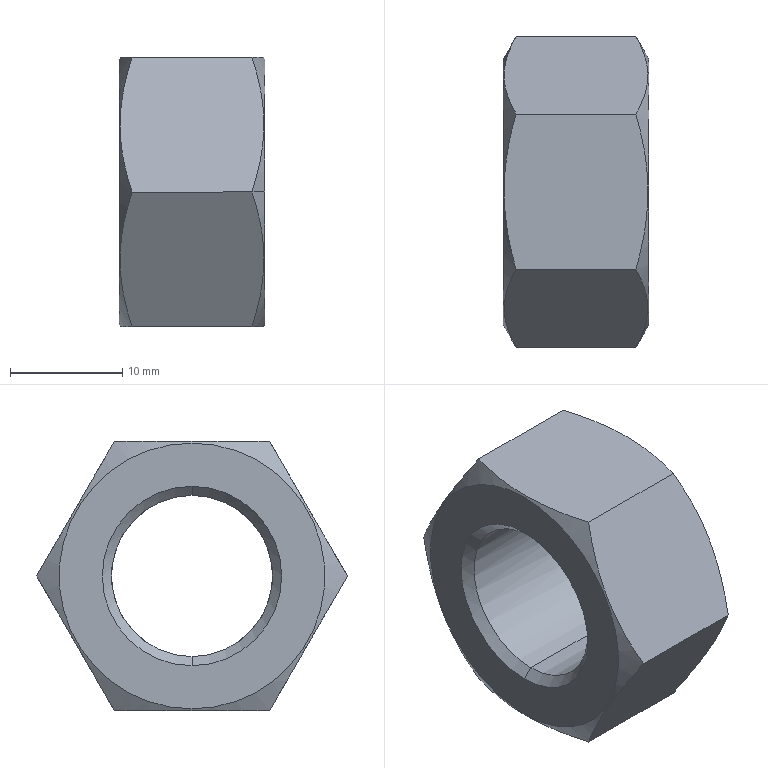Part | SolidWorks | features BaseBody 1 | 1 solid | 18 faces | box 13 x 27.713 x 24 mm | volume 4305 mm3 | cone 8 | plane 8 | cylinder 2 | commonest cylinder face diameters 14.376 x2
STEP:
#1=CARTESIAN_POINT('',(12.188,0.,-7.188));
#2=VERTEX_POINT('',#1);
#3=CARTESIAN_POINT('',(12.188,-7.188,0.));
#4=VERTEX_POINT('',#3);
#5=CARTESIAN_POINT('',(12.188,0.,0.));
#6=DIRECTION('',(-1.,0.,0.));
#7=DIRECTION('',(0.,0.,1.));
#8=AXIS2_PLACEMENT_3D('',#5,#6,#7);
#9=CIRCLE('',#8,7.188);
#10=EDGE_CURVE('',#2,#4,#9,.T.);
#11=ORIENTED_EDGE('',*,*,#10,.F.);
#12=CARTESIAN_POINT('',(0.812,0.,-7.188));
#13=VERTEX_POINT('',#12);
#14=CARTESIAN_POINT('',(13.,0.,-7.188));
#15=DIRECTION('',(-1.,0.,0.));
#16=VECTOR('',#15,1000.);
#17=LINE('',#14,#16);
#18=EDGE_CURVE('',#2,#13,#17,.T.);
#19=ORIENTED_EDGE('',*,*,#18,.T.);
#20=CARTESIAN_POINT('',(0.812,0.,7.188));
#21=VERTEX_POINT('',#20);
#22=CARTESIAN_POINT('',(0.812,0.,0.));
#23=DIRECTION('',(1.,0.,0.));
#24=DIRECTION('',(0.,0.,1.));
#25=AXIS2_PLACEMENT_3D('',#22,#23,#24);
#26=CIRCLE('',#25,7.188);
#27=EDGE_CURVE('',#21,#13,#26,.T.);
#28=ORIENTED_EDGE('',*,*,#27,.F.);
#29=CARTESIAN_POINT('',(12.188,0.,7.188));
#30=VERTEX_POINT('',#29);
#31=CARTESIAN_POINT('',(13.,0.,7.188));
#32=DIRECTION('',(-1.,0.,0.));
#33=VECTOR('',#32,1000.);
#34=LINE('',#31,#33);
#35=EDGE_CURVE('',#30,#21,#34,.T.);
#36=ORIENTED_EDGE('',*,*,#35,.F.);
#37=CARTESIAN_POINT('',(12.188,0.,0.));
#38=DIRECTION('',(-1.,0.,0.));
#39=DIRECTION('',(0.,0.,1.));
#40=AXIS2_PLACEMENT_3D('',#37,#38,#39);
#41=CIRCLE('',#40,7.188);
#42=EDGE_CURVE('',#4,#30,#41,.T.);
#43=ORIENTED_EDGE('',*,*,#42,.F.);
#44=EDGE_LOOP('',(#11,#19,#28,#36,#43));
#45=FACE_OUTER_BOUND('',#44,.T.);
#46=CARTESIAN_POINT('',(13.,0.,0.));
#47=DIRECTION('',(-1.,0.,0.));
#48=DIRECTION('',(0.,0.,1.));
#49=AXIS2_PLACEMENT_3D('',#46,#47,#48);
#50=CYLINDRICAL_SURFACE('',#49,7.188);
#51=ADVANCED_FACE('',(#45),#50,.F.);
#52=ORIENTED_EDGE('',*,*,#27,.T.);
#53=CARTESIAN_POINT('',(0.,0.,-8.));
#54=VERTEX_POINT('',#53);
#55=CARTESIAN_POINT('',(0.,0.,-8.));
#56=DIRECTION('',(-0.7071,0.,-0.7071));
#57=VECTOR('',#56,1000.);
#58=LINE('',#55,#57);
#59=EDGE_CURVE('',#13,#54,#58,.T.);
#60=ORIENTED_EDGE('',*,*,#59,.T.);
#61=CARTESIAN_POINT('',(0.,0.,8.));
#62=VERTEX_POINT('',#61);
#63=CARTESIAN_POINT('',(0.,0.,0.));
#64=DIRECTION('',(1.,0.,0.));
#65=DIRECTION('',(0.,0.,1.));
#66=AXIS2_PLACEMENT_3D('',#63,#64,#65);
#67=CIRCLE('',#66,8.);
#68=EDGE_CURVE('',#62,#54,#67,.T.);
#69=ORIENTED_EDGE('',*,*,#68,.F.);
#70=CARTESIAN_POINT('',(0.,0.,8.));
#71=DIRECTION('',(-0.7071,0.,0.7071));
#72=VECTOR('',#71,1000.);
#73=LINE('',#70,#72);
#74=EDGE_CURVE('',#21,#62,#73,.T.);
#75=ORIENTED_EDGE('',*,*,#74,.F.);
#76=EDGE_LOOP('',(#52,#60,#69,#75));
#77=FACE_OUTER_BOUND('',#76,.T.);
#78=CARTESIAN_POINT('',(0.,0.,0.));
#79=DIRECTION('',(-1.,0.,0.));
#80=DIRECTION('',(0.,0.,1.));
#81=AXIS2_PLACEMENT_3D('',#78,#79,#80);
#82=CONICAL_SURFACE('',#81,8.,0.7854);
#83=ADVANCED_FACE('',(#77),#82,.F.);
#84=CARTESIAN_POINT('',(12.188,7.188,0.));
#85=VERTEX_POINT('',#84);
#86=CARTESIAN_POINT('',(12.188,0.,0.));
#87=DIRECTION('',(-1.,0.,0.));
#88=DIRECTION('',(0.,0.,1.));
#89=AXIS2_PLACEMENT_3D('',#86,#87,#88);
#90=CIRCLE('',#89,7.188);
#91=EDGE_CURVE('',#85,#2,#90,.T.);
#92=ORIENTED_EDGE('',*,*,#91,.T.);
#93=ORIENTED_EDGE('',*,*,#10,.T.);
#94=CARTESIAN_POINT('',(13.,-8.,0.));
#95=VERTEX_POINT('',#94);
#96=CARTESIAN_POINT('',(13.,-8.,0.));
#97=DIRECTION('',(0.7071,-0.7071,0.));
#98=VECTOR('',#97,1000.);
#99=LINE('',#96,#98);
#100=EDGE_CURVE('',#4,#95,#99,.T.);
#101=ORIENTED_EDGE('',*,*,#100,.T.);
#102=CARTESIAN_POINT('',(13.,8.,0.));
#103=VERTEX_POINT('',#102);
#104=CARTESIAN_POINT('',(13.,0.,0.));
#105=DIRECTION('',(-1.,0.,0.));
#106=DIRECTION('',(0.,1.,0.));
#107=AXIS2_PLACEMENT_3D('',#104,#105,#106);
#108=CIRCLE('',#107,8.);
#109=EDGE_CURVE('',#103,#95,#108,.T.);
#110=ORIENTED_EDGE('',*,*,#109,.F.);
#111=CARTESIAN_POINT('',(13.,8.,0.));
#112=DIRECTION('',(0.7071,0.7071,0.));
#113=VECTOR('',#112,1000.);
#114=LINE('',#111,#113);
#115=EDGE_CURVE('',#85,#103,#114,.T.);
#116=ORIENTED_EDGE('',*,*,#115,.F.);
#117=EDGE_LOOP('',(#92,#93,#101,#110,#116));
#118=FACE_OUTER_BOUND('',#117,.T.);
#119=CARTESIAN_POINT('',(13.,0.,0.));
#120=DIRECTION('',(1.,0.,0.));
#121=DIRECTION('',(0.,1.,0.));
#122=AXIS2_PLACEMENT_3D('',#119,#120,#121);
#123=CONICAL_SURFACE('',#122,8.,0.7854);
#124=ADVANCED_FACE('',(#118),#123,.F.);
#125=CARTESIAN_POINT('',(0.,0.,-11.85));
#126=VERTEX_POINT('',#125);
#127=CARTESIAN_POINT('',(0.,0.,11.85));
#128=VERTEX_POINT('',#127);
#129=CARTESIAN_POINT('',(0.,0.,0.));
#130=DIRECTION('',(1.,0.,0.));
#131=DIRECTION('',(0.,0.,-1.));
#132=AXIS2_PLACEMENT_3D('',#129,#130,#131);
#133=CIRCLE('',#132,11.85);
#134=EDGE_CURVE('',#126,#128,#133,.T.);
#135=ORIENTED_EDGE('',*,*,#134,.T.);
#136=CARTESIAN_POINT('',(0.0866,0.,12.));
#137=VERTEX_POINT('',#136);
#138=CARTESIAN_POINT('',(1.165,0.,13.868));
#139=DIRECTION('',(0.5,0.,0.866));
#140=VECTOR('',#139,1000.);
#141=LINE('',#138,#140);
#142=EDGE_CURVE('',#128,#137,#141,.T.);
#143=ORIENTED_EDGE('',*,*,#142,.T.);
#144=CARTESIAN_POINT('',(1.158,6.928,12.));
#145=VERTEX_POINT('',#144);
#146=CARTESIAN_POINT('',(0.0866,0.,12.));
#147=CARTESIAN_POINT('',(0.0866,0.588,12.));
#148=CARTESIAN_POINT('',(0.1119,1.179,12.));
#149=CARTESIAN_POINT('',(0.21,2.347,12.));
#150=CARTESIAN_POINT('',(0.2826,2.927,12.));
#151=CARTESIAN_POINT('',(0.5626,4.658,12.));
#152=CARTESIAN_POINT('',(0.832,5.798,12.));
#153=CARTESIAN_POINT('',(1.158,6.928,12.));
#154=B_SPLINE_CURVE_WITH_KNOTS('',3,(#146,#147,#148,#149,#150,#151,#152,#153),.UNSPECIFIED.,.F.,.F.,(4,2,2,4),(0.00701,0.008756,0.0105,0.01399),.UNSPECIFIED.);
#155=EDGE_CURVE('',#137,#145,#154,.T.);
#156=ORIENTED_EDGE('',*,*,#155,.T.);
#157=CARTESIAN_POINT('',(1.158,13.856,0.000000037));
#158=VERTEX_POINT('',#157);
#159=CARTESIAN_POINT('',(1.158,6.928,12.));
#160=CARTESIAN_POINT('',(0.8318,7.494,11.02));
#161=CARTESIAN_POINT('',(0.5627,8.064,10.033));
#162=CARTESIAN_POINT('',(0.1898,9.215,8.039));
#163=CARTESIAN_POINT('',(0.08736,9.797,7.032));
#164=CARTESIAN_POINT('',(0.08623,10.68,5.501));
#165=CARTESIAN_POINT('',(0.1113,10.976,4.989));
#166=CARTESIAN_POINT('',(0.209,11.561,3.975));
#167=CARTESIAN_POINT('',(0.2815,11.852,3.472));
#168=CARTESIAN_POINT('',(0.5616,12.719,1.97));
#169=CARTESIAN_POINT('',(0.8314,13.29,0.9809));
#170=CARTESIAN_POINT('',(1.158,13.856,0.000000037));
#171=B_SPLINE_CURVE_WITH_KNOTS('',3,(#159,#160,#161,#162,#163,#164,#165,#166,#167,#168,#169,#170),.UNSPECIFIED.,.F.,.F.,(4,2,2,2,2,4),(0.,0.003499,0.006997,0.008746,0.0105,0.01399),.UNSPECIFIED.);
#172=EDGE_CURVE('',#145,#158,#171,.T.);
#173=ORIENTED_EDGE('',*,*,#172,.T.);
#174=CARTESIAN_POINT('',(1.158,6.928,-12.));
#175=VERTEX_POINT('',#174);
#176=CARTESIAN_POINT('',(1.158,13.856,0.000000037));
#177=CARTESIAN_POINT('',(0.8318,13.291,-0.9797));
#178=CARTESIAN_POINT('',(0.5627,12.721,-1.967));
#179=CARTESIAN_POINT('',(0.1898,11.57,-3.961));
#180=CARTESIAN_POINT('',(0.08736,10.988,-4.968));
#181=CARTESIAN_POINT('',(0.08623,10.104,-6.499));
#182=CARTESIAN_POINT('',(0.1113,9.809,-7.011));
#183=CARTESIAN_POINT('',(0.209,9.223,-8.025));
#184=CARTESIAN_POINT('',(0.2815,8.933,-8.528));
#185=CARTESIAN_POINT('',(0.5616,8.066,-10.03));
#186=CARTESIAN_POINT('',(0.8314,7.495,-11.019));
#187=CARTESIAN_POINT('',(1.158,6.928,-12.));
#188=B_SPLINE_CURVE_WITH_KNOTS('',3,(#176,#177,#178,#179,#180,#181,#182,#183,#184,#185,#186,#187),.UNSPECIFIED.,.F.,.F.,(4,2,2,2,2,4),(0.,0.003499,0.006997,0.008746,0.0105,0.01399),.UNSPECIFIED.);
#189=EDGE_CURVE('',#158,#175,#188,.T.);
#190=ORIENTED_EDGE('',*,*,#189,.T.);
#191=CARTESIAN_POINT('',(0.0866,0.,-12.));
#192=VERTEX_POINT('',#191);
#193=CARTESIAN_POINT('',(1.158,6.928,-12.));
#194=CARTESIAN_POINT('',(0.8312,5.795,-12.));
#195=CARTESIAN_POINT('',(0.5617,4.653,-12.));
#196=CARTESIAN_POINT('',(0.1888,2.346,-12.));
#197=CARTESIAN_POINT('',(0.0866,1.18,-12.));
#198=CARTESIAN_POINT('',(0.0866,0.,-12.));
#199=B_SPLINE_CURVE_WITH_KNOTS('',3,(#193,#194,#195,#196,#197,#198),.UNSPECIFIED.,.F.,.F.,(4,2,4),(0.,0.003505,0.00701),.UNSPECIFIED.);
#200=EDGE_CURVE('',#175,#192,#199,.T.);
#201=ORIENTED_EDGE('',*,*,#200,.T.);
#202=CARTESIAN_POINT('',(1.165,0.,-13.868));
#203=DIRECTION('',(0.5,0.,-0.866));
#204=VECTOR('',#203,1000.);
#205=LINE('',#202,#204);
#206=EDGE_CURVE('',#126,#192,#205,.T.);
#207=ORIENTED_EDGE('',*,*,#206,.F.);
#208=EDGE_LOOP('',(#135,#143,#156,#173,#190,#201,#207));
#209=FACE_OUTER_BOUND('',#208,.T.);
#210=CARTESIAN_POINT('',(1.165,0.,0.));
#211=DIRECTION('',(1.,0.,0.));
#212=DIRECTION('',(0.,0.,-1.));
#213=AXIS2_PLACEMENT_3D('',#210,#211,#212);
#214=CONICAL_SURFACE('',#213,13.868,1.047);
#215=ADVANCED_FACE('',(#209),#214,.T.);
#216=CARTESIAN_POINT('',(13.,-11.85,0.));
#217=VERTEX_POINT('',#216);
#218=CARTESIAN_POINT('',(13.,11.85,0.));
#219=VERTEX_POINT('',#218);
#220=CARTESIAN_POINT('',(13.,0.,0.));
#221=DIRECTION('',(-1.,0.,0.));
#222=DIRECTION('',(0.,-1.,0.));
#223=AXIS2_PLACEMENT_3D('',#220,#221,#222);
#224=CIRCLE('',#223,11.85);
#225=EDGE_CURVE('',#217,#219,#224,.T.);
#226=ORIENTED_EDGE('',*,*,#225,.T.);
#227=CARTESIAN_POINT('',(11.842,13.856,0.000000014));
#228=VERTEX_POINT('',#227);
#229=CARTESIAN_POINT('',(11.835,13.868,0.));
#230=DIRECTION('',(-0.5,0.866,0.));
#231=VECTOR('',#230,1000.);
#232=LINE('',#229,#231);
#233=EDGE_CURVE('',#219,#228,#232,.T.);
#234=ORIENTED_EDGE('',*,*,#233,.T.);
#235=CARTESIAN_POINT('',(11.842,6.928,12.));
#236=VERTEX_POINT('',#235);
#237=CARTESIAN_POINT('',(11.842,13.856,0.000000014));
#238=CARTESIAN_POINT('',(12.168,13.291,0.9797));
#239=CARTESIAN_POINT('',(12.437,12.721,1.967));
#240=CARTESIAN_POINT('',(12.81,11.57,3.961));
#241=CARTESIAN_POINT('',(12.913,10.988,4.968));
#242=CARTESIAN_POINT('',(12.914,10.104,6.499));
#243=CARTESIAN_POINT('',(12.889,9.809,7.011));
#244=CARTESIAN_POINT('',(12.791,9.223,8.025));
#245=CARTESIAN_POINT('',(12.718,8.933,8.528));
#246=CARTESIAN_POINT('',(12.438,8.066,10.03));
#247=CARTESIAN_POINT('',(12.169,7.495,11.019));
#248=CARTESIAN_POINT('',(11.842,6.928,12.));
#249=B_SPLINE_CURVE_WITH_KNOTS('',3,(#237,#238,#239,#240,#241,#242,#243,#244,#245,#246,#247,#248),.UNSPECIFIED.,.F.,.F.,(4,2,2,2,2,4),(0.,0.003499,0.006997,0.008746,0.0105,0.01399),.UNSPECIFIED.);
#250=EDGE_CURVE('',#228,#236,#249,.T.);
#251=ORIENTED_EDGE('',*,*,#250,.T.);
#252=CARTESIAN_POINT('',(11.842,-6.928,12.));
#253=VERTEX_POINT('',#252);
#254=CARTESIAN_POINT('',(11.842,6.928,12.));
#255=CARTESIAN_POINT('',(12.168,5.797,12.));
#256=CARTESIAN_POINT('',(12.437,4.657,12.));
#257=CARTESIAN_POINT('',(12.81,2.355,12.));
#258=CARTESIAN_POINT('',(12.913,1.191,12.));
#259=CARTESIAN_POINT('',(12.914,-0.5758,12.));
#260=CARTESIAN_POINT('',(12.889,-1.168,12.));
#261=CARTESIAN_POINT('',(12.791,-2.338,12.));
#262=CARTESIAN_POINT('',(12.718,-2.92,12.));
#263=CARTESIAN_POINT('',(12.438,-4.653,12.));
#264=CARTESIAN_POINT('',(12.169,-5.796,12.));
#265=CARTESIAN_POINT('',(11.842,-6.928,12.));
#266=B_SPLINE_CURVE_WITH_KNOTS('',3,(#254,#255,#256,#257,#258,#259,#260,#261,#262,#263,#264,#265),.UNSPECIFIED.,.F.,.F.,(4,2,2,2,2,4),(0.,0.003499,0.006997,0.008746,0.0105,0.01399),.UNSPECIFIED.);
#267=EDGE_CURVE('',#236,#253,#266,.T.);
#268=ORIENTED_EDGE('',*,*,#267,.T.);
#269=CARTESIAN_POINT('',(11.842,-13.856,0.000000012));
#270=VERTEX_POINT('',#269);
#271=CARTESIAN_POINT('',(11.842,-6.928,12.));
#272=CARTESIAN_POINT('',(12.168,-7.494,11.02));
#273=CARTESIAN_POINT('',(12.437,-8.064,10.033));
#274=CARTESIAN_POINT('',(12.81,-9.215,8.039));
#275=CARTESIAN_POINT('',(12.913,-9.797,7.032));
#276=CARTESIAN_POINT('',(12.914,-10.68,5.501));
#277=CARTESIAN_POINT('',(12.889,-10.976,4.989));
#278=CARTESIAN_POINT('',(12.791,-11.561,3.975));
#279=CARTESIAN_POINT('',(12.718,-11.852,3.472));
#280=CARTESIAN_POINT('',(12.438,-12.719,1.97));
#281=CARTESIAN_POINT('',(12.169,-13.29,0.9809));
#282=CARTESIAN_POINT('',(11.842,-13.856,0.000000012));
#283=B_SPLINE_CURVE_WITH_KNOTS('',3,(#271,#272,#273,#274,#275,#276,#277,#278,#279,#280,#281,#282),.UNSPECIFIED.,.F.,.F.,(4,2,2,2,2,4),(0.,0.003499,0.006997,0.008746,0.0105,0.01399),.UNSPECIFIED.);
#284=EDGE_CURVE('',#253,#270,#283,.T.);
#285=ORIENTED_EDGE('',*,*,#284,.T.);
#286=CARTESIAN_POINT('',(11.835,-13.868,0.));
#287=DIRECTION('',(-0.5,-0.866,0.));
#288=VECTOR('',#287,1000.);
#289=LINE('',#286,#288);
#290=EDGE_CURVE('',#217,#270,#289,.T.);
#291=ORIENTED_EDGE('',*,*,#290,.F.);
#292=EDGE_LOOP('',(#226,#234,#251,#268,#285,#291));
#293=FACE_OUTER_BOUND('',#292,.T.);
#294=CARTESIAN_POINT('',(11.835,0.,0.));
#295=DIRECTION('',(-1.,0.,0.));
#296=DIRECTION('',(0.,-1.,0.));
#297=AXIS2_PLACEMENT_3D('',#294,#295,#296);
#298=CONICAL_SURFACE('',#297,13.868,1.047);
#299=ADVANCED_FACE('',(#293),#298,.T.);
#300=ORIENTED_EDGE('',*,*,#18,.F.);
#301=ORIENTED_EDGE('',*,*,#91,.F.);
#302=CARTESIAN_POINT('',(12.188,0.,0.));
#303=DIRECTION('',(-1.,0.,0.));
#304=DIRECTION('',(0.,0.,1.));
#305=AXIS2_PLACEMENT_3D('',#302,#303,#304);
#306=CIRCLE('',#305,7.188);
#307=EDGE_CURVE('',#30,#85,#306,.T.);
#308=ORIENTED_EDGE('',*,*,#307,.F.);
#309=ORIENTED_EDGE('',*,*,#35,.T.);
#310=CARTESIAN_POINT('',(0.812,0.,0.));
#311=DIRECTION('',(1.,0.,0.));
#312=DIRECTION('',(0.,0.,1.));
#313=AXIS2_PLACEMENT_3D('',#310,#311,#312);
#314=CIRCLE('',#313,7.188);
#315=EDGE_CURVE('',#13,#21,#314,.T.);
#316=ORIENTED_EDGE('',*,*,#315,.F.);
#317=EDGE_LOOP('',(#300,#301,#308,#309,#316));
#318=FACE_OUTER_BOUND('',#317,.T.);
#319=CARTESIAN_POINT('',(13.,0.,0.));
#320=DIRECTION('',(-1.,0.,0.));
#321=DIRECTION('',(0.,0.,1.));
#322=AXIS2_PLACEMENT_3D('',#319,#320,#321);
#323=CYLINDRICAL_SURFACE('',#322,7.188);
#324=ADVANCED_FACE('',(#318),#323,.F.);
#325=ORIENTED_EDGE('',*,*,#59,.F.);
#326=ORIENTED_EDGE('',*,*,#315,.T.);
#327=ORIENTED_EDGE('',*,*,#74,.T.);
#328=CARTESIAN_POINT('',(0.,0.,0.));
#329=DIRECTION('',(1.,0.,0.));
#330=DIRECTION('',(0.,0.,1.));
#331=AXIS2_PLACEMENT_3D('',#328,#329,#330);
#332=CIRCLE('',#331,8.);
#333=EDGE_CURVE('',#54,#62,#332,.T.);
#334=ORIENTED_EDGE('',*,*,#333,.F.);
#335=EDGE_LOOP('',(#325,#326,#327,#334));
#336=FACE_OUTER_BOUND('',#335,.T.);
#337=CARTESIAN_POINT('',(0.,0.,0.));
#338=DIRECTION('',(-1.,0.,0.));
#339=DIRECTION('',(0.,0.,1.));
#340=AXIS2_PLACEMENT_3D('',#337,#338,#339);
#341=CONICAL_SURFACE('',#340,8.,0.7854);
#342=ADVANCED_FACE('',(#336),#341,.F.);
#343=ORIENTED_EDGE('',*,*,#100,.F.);
#344=ORIENTED_EDGE('',*,*,#42,.T.);
#345=ORIENTED_EDGE('',*,*,#307,.T.);
#346=ORIENTED_EDGE('',*,*,#115,.T.);
#347=CARTESIAN_POINT('',(13.,0.,0.));
#348=DIRECTION('',(-1.,0.,0.));
#349=DIRECTION('',(0.,1.,0.));
#350=AXIS2_PLACEMENT_3D('',#347,#348,#349);
#351=CIRCLE('',#350,8.);
#352=EDGE_CURVE('',#95,#103,#351,.T.);
#353=ORIENTED_EDGE('',*,*,#352,.F.);
#354=EDGE_LOOP('',(#343,#344,#345,#346,#353));
#355=FACE_OUTER_BOUND('',#354,.T.);
#356=CARTESIAN_POINT('',(13.,0.,0.));
#357=DIRECTION('',(1.,0.,0.));
#358=DIRECTION('',(0.,1.,0.));
#359=AXIS2_PLACEMENT_3D('',#356,#357,#358);
#360=CONICAL_SURFACE('',#359,8.,0.7854);
#361=ADVANCED_FACE('',(#355),#360,.F.);
#362=ORIENTED_EDGE('',*,*,#68,.T.);
#363=ORIENTED_EDGE('',*,*,#333,.T.);
#364=EDGE_LOOP('',(#362,#363));
#365=FACE_BOUND('',#364,.T.);
#366=ORIENTED_EDGE('',*,*,#134,.F.);
#367=CARTESIAN_POINT('',(0.,0.,0.));
#368=DIRECTION('',(1.,0.,0.));
#369=DIRECTION('',(0.,0.,-1.));
#370=AXIS2_PLACEMENT_3D('',#367,#368,#369);
#371=CIRCLE('',#370,11.85);
#372=EDGE_CURVE('',#128,#126,#371,.T.);
#373=ORIENTED_EDGE('',*,*,#372,.F.);
#374=EDGE_LOOP('',(#366,#373));
#375=FACE_OUTER_BOUND('',#374,.T.);
#376=CARTESIAN_POINT('',(0.,0.,0.));
#377=DIRECTION('',(1.,0.,0.));
#378=DIRECTION('',(0.,0.,-1.));
#379=AXIS2_PLACEMENT_3D('',#376,#377,#378);
#380=PLANE('',#379);
#381=ADVANCED_FACE('',(#365,#375),#380,.F.);
#382=ORIENTED_EDGE('',*,*,#225,.F.);
#383=CARTESIAN_POINT('',(13.,0.,0.));
#384=DIRECTION('',(-1.,0.,0.));
#385=DIRECTION('',(0.,-1.,0.));
#386=AXIS2_PLACEMENT_3D('',#383,#384,#385);
#387=CIRCLE('',#386,11.85);
#388=EDGE_CURVE('',#219,#217,#387,.T.);
#389=ORIENTED_EDGE('',*,*,#388,.F.);
#390=EDGE_LOOP('',(#382,#389));
#391=FACE_OUTER_BOUND('',#390,.T.);
#392=ORIENTED_EDGE('',*,*,#109,.T.);
#393=ORIENTED_EDGE('',*,*,#352,.T.);
#394=EDGE_LOOP('',(#392,#393));
#395=FACE_BOUND('',#394,.T.);
#396=CARTESIAN_POINT('',(13.,11.85,0.));
#397=DIRECTION('',(-1.,0.,0.));
#398=DIRECTION('',(0.,0.,1.));
#399=AXIS2_PLACEMENT_3D('',#396,#397,#398);
#400=PLANE('',#399);
#401=ADVANCED_FACE('',(#391,#395),#400,.F.);
#402=ORIENTED_EDGE('',*,*,#142,.F.);
#403=ORIENTED_EDGE('',*,*,#372,.T.);
#404=ORIENTED_EDGE('',*,*,#206,.T.);
#405=CARTESIAN_POINT('',(1.158,-6.928,-12.));
#406=VERTEX_POINT('',#405);
#407=CARTESIAN_POINT('',(0.0866,0.,-12.));
#408=CARTESIAN_POINT('',(0.0866,-0.588,-12.));
#409=CARTESIAN_POINT('',(0.1119,-1.179,-12.));
#410=CARTESIAN_POINT('',(0.21,-2.347,-12.));
#411=CARTESIAN_POINT('',(0.2826,-2.927,-12.));
#412=CARTESIAN_POINT('',(0.5626,-4.658,-12.));
#413=CARTESIAN_POINT('',(0.832,-5.798,-12.));
#414=CARTESIAN_POINT('',(1.158,-6.928,-12.));
#415=B_SPLINE_CURVE_WITH_KNOTS('',3,(#407,#408,#409,#410,#411,#412,#413,#414),.UNSPECIFIED.,.F.,.F.,(4,2,2,4),(0.00701,0.008756,0.0105,0.01399),.UNSPECIFIED.);
#416=EDGE_CURVE('',#192,#406,#415,.T.);
#417=ORIENTED_EDGE('',*,*,#416,.T.);
#418=CARTESIAN_POINT('',(1.158,-13.856,-0.000000037));
#419=VERTEX_POINT('',#418);
#420=CARTESIAN_POINT('',(1.158,-6.928,-12.));
#421=CARTESIAN_POINT('',(0.8318,-7.494,-11.02));
#422=CARTESIAN_POINT('',(0.5627,-8.064,-10.033));
#423=CARTESIAN_POINT('',(0.1898,-9.215,-8.039));
#424=CARTESIAN_POINT('',(0.08736,-9.797,-7.032));
#425=CARTESIAN_POINT('',(0.08623,-10.68,-5.501));
#426=CARTESIAN_POINT('',(0.1113,-10.976,-4.989));
#427=CARTESIAN_POINT('',(0.209,-11.561,-3.975));
#428=CARTESIAN_POINT('',(0.2815,-11.852,-3.472));
#429=CARTESIAN_POINT('',(0.5616,-12.719,-1.97));
#430=CARTESIAN_POINT('',(0.8314,-13.29,-0.9809));
#431=CARTESIAN_POINT('',(1.158,-13.856,-0.000000037));
#432=B_SPLINE_CURVE_WITH_KNOTS('',3,(#420,#421,#422,#423,#424,#425,#426,#427,#428,#429,#430,#431),.UNSPECIFIED.,.F.,.F.,(4,2,2,2,2,4),(0.,0.003499,0.006997,0.008746,0.0105,0.01399),.UNSPECIFIED.);
#433=EDGE_CURVE('',#406,#419,#432,.T.);
#434=ORIENTED_EDGE('',*,*,#433,.T.);
#435=CARTESIAN_POINT('',(1.158,-6.928,12.));
#436=VERTEX_POINT('',#435);
#437=CARTESIAN_POINT('',(1.158,-13.856,-0.000000037));
#438=CARTESIAN_POINT('',(0.8318,-13.291,0.9797));
#439=CARTESIAN_POINT('',(0.5627,-12.721,1.967));
#440=CARTESIAN_POINT('',(0.1898,-11.57,3.961));
#441=CARTESIAN_POINT('',(0.08736,-10.988,4.968));
#442=CARTESIAN_POINT('',(0.08623,-10.104,6.499));
#443=CARTESIAN_POINT('',(0.1113,-9.809,7.011));
#444=CARTESIAN_POINT('',(0.209,-9.223,8.025));
#445=CARTESIAN_POINT('',(0.2815,-8.933,8.528));
#446=CARTESIAN_POINT('',(0.5616,-8.066,10.03));
#447=CARTESIAN_POINT('',(0.8314,-7.495,11.019));
#448=CARTESIAN_POINT('',(1.158,-6.928,12.));
#449=B_SPLINE_CURVE_WITH_KNOTS('',3,(#437,#438,#439,#440,#441,#442,#443,#444,#445,#446,#447,#448),.UNSPECIFIED.,.F.,.F.,(4,2,2,2,2,4),(0.,0.003499,0.006997,0.008746,0.0105,0.01399),.UNSPECIFIED.);
#450=EDGE_CURVE('',#419,#436,#449,.T.);
#451=ORIENTED_EDGE('',*,*,#450,.T.);
#452=CARTESIAN_POINT('',(1.158,-6.928,12.));
#453=CARTESIAN_POINT('',(0.8312,-5.795,12.));
#454=CARTESIAN_POINT('',(0.5617,-4.653,12.));
#455=CARTESIAN_POINT('',(0.1888,-2.346,12.));
#456=CARTESIAN_POINT('',(0.0866,-1.18,12.));
#457=CARTESIAN_POINT('',(0.0866,0.,12.));
#458=B_SPLINE_CURVE_WITH_KNOTS('',3,(#452,#453,#454,#455,#456,#457),.UNSPECIFIED.,.F.,.F.,(4,2,4),(0.,0.003505,0.00701),.UNSPECIFIED.);
#459=EDGE_CURVE('',#436,#137,#458,.T.);
#460=ORIENTED_EDGE('',*,*,#459,.T.);
#461=EDGE_LOOP('',(#402,#403,#404,#417,#434,#451,#460));
#462=FACE_OUTER_BOUND('',#461,.T.);
#463=CARTESIAN_POINT('',(1.165,0.,0.));
#464=DIRECTION('',(1.,0.,0.));
#465=DIRECTION('',(0.,0.,-1.));
#466=AXIS2_PLACEMENT_3D('',#463,#464,#465);
#467=CONICAL_SURFACE('',#466,13.868,1.047);
#468=ADVANCED_FACE('',(#462),#467,.T.);
#469=ORIENTED_EDGE('',*,*,#233,.F.);
#470=ORIENTED_EDGE('',*,*,#388,.T.);
#471=ORIENTED_EDGE('',*,*,#290,.T.);
#472=CARTESIAN_POINT('',(11.842,-6.928,-12.));
#473=VERTEX_POINT('',#472);
#474=CARTESIAN_POINT('',(11.842,-13.856,0.000000012));
#475=CARTESIAN_POINT('',(12.168,-13.291,-0.9797));
#476=CARTESIAN_POINT('',(12.437,-12.721,-1.967));
#477=CARTESIAN_POINT('',(12.81,-11.57,-3.961));
#478=CARTESIAN_POINT('',(12.913,-10.988,-4.968));
#479=CARTESIAN_POINT('',(12.914,-10.104,-6.499));
#480=CARTESIAN_POINT('',(12.889,-9.809,-7.011));
#481=CARTESIAN_POINT('',(12.791,-9.223,-8.025));
#482=CARTESIAN_POINT('',(12.718,-8.933,-8.528));
#483=CARTESIAN_POINT('',(12.438,-8.066,-10.03));
#484=CARTESIAN_POINT('',(12.169,-7.495,-11.019));
#485=CARTESIAN_POINT('',(11.842,-6.928,-12.));
#486=B_SPLINE_CURVE_WITH_KNOTS('',3,(#474,#475,#476,#477,#478,#479,#480,#481,#482,#483,#484,#485),.UNSPECIFIED.,.F.,.F.,(4,2,2,2,2,4),(0.,0.003499,0.006997,0.008746,0.0105,0.01399),.UNSPECIFIED.);
#487=EDGE_CURVE('',#270,#473,#486,.T.);
#488=ORIENTED_EDGE('',*,*,#487,.T.);
#489=CARTESIAN_POINT('',(11.842,6.928,-12.));
#490=VERTEX_POINT('',#489);
#491=CARTESIAN_POINT('',(11.842,-6.928,-12.));
#492=CARTESIAN_POINT('',(12.168,-5.797,-12.));
#493=CARTESIAN_POINT('',(12.437,-4.657,-12.));
#494=CARTESIAN_POINT('',(12.81,-2.355,-12.));
#495=CARTESIAN_POINT('',(12.913,-1.191,-12.));
#496=CARTESIAN_POINT('',(12.914,0.5758,-12.));
#497=CARTESIAN_POINT('',(12.889,1.168,-12.));
#498=CARTESIAN_POINT('',(12.791,2.338,-12.));
#499=CARTESIAN_POINT('',(12.718,2.92,-12.));
#500=CARTESIAN_POINT('',(12.438,4.653,-12.));
#501=CARTESIAN_POINT('',(12.169,5.796,-12.));
#502=CARTESIAN_POINT('',(11.842,6.928,-12.));
#503=B_SPLINE_CURVE_WITH_KNOTS('',3,(#491,#492,#493,#494,#495,#496,#497,#498,#499,#500,#501,#502),.UNSPECIFIED.,.F.,.F.,(4,2,2,2,2,4),(0.,0.003499,0.006997,0.008746,0.0105,0.01399),.UNSPECIFIED.);
#504=EDGE_CURVE('',#473,#490,#503,.T.);
#505=ORIENTED_EDGE('',*,*,#504,.T.);
#506=CARTESIAN_POINT('',(11.842,6.928,-12.));
#507=CARTESIAN_POINT('',(12.168,7.494,-11.02));
#508=CARTESIAN_POINT('',(12.437,8.064,-10.033));
#509=CARTESIAN_POINT('',(12.81,9.215,-8.039));
#510=CARTESIAN_POINT('',(12.913,9.797,-7.032));
#511=CARTESIAN_POINT('',(12.914,10.68,-5.501));
#512=CARTESIAN_POINT('',(12.889,10.976,-4.989));
#513=CARTESIAN_POINT('',(12.791,11.561,-3.975));
#514=CARTESIAN_POINT('',(12.718,11.852,-3.472));
#515=CARTESIAN_POINT('',(12.438,12.719,-1.97));
#516=CARTESIAN_POINT('',(12.169,13.29,-0.9809));
#517=CARTESIAN_POINT('',(11.842,13.856,0.000000014));
#518=B_SPLINE_CURVE_WITH_KNOTS('',3,(#506,#507,#508,#509,#510,#511,#512,#513,#514,#515,#516,#517),.UNSPECIFIED.,.F.,.F.,(4,2,2,2,2,4),(0.,0.003499,0.006997,0.008746,0.0105,0.01399),.UNSPECIFIED.);
#519=EDGE_CURVE('',#490,#228,#518,.T.);
#520=ORIENTED_EDGE('',*,*,#519,.T.);
#521=EDGE_LOOP('',(#469,#470,#471,#488,#505,#520));
#522=FACE_OUTER_BOUND('',#521,.T.);
#523=CARTESIAN_POINT('',(11.835,0.,0.));
#524=DIRECTION('',(-1.,0.,0.));
#525=DIRECTION('',(0.,-1.,0.));
#526=AXIS2_PLACEMENT_3D('',#523,#524,#525);
#527=CONICAL_SURFACE('',#526,13.868,1.047);
#528=ADVANCED_FACE('',(#522),#527,.T.);
#529=ORIENTED_EDGE('',*,*,#267,.F.);
#530=CARTESIAN_POINT('',(13.,6.928,12.));
#531=DIRECTION('',(1.,0.,0.));
#532=VECTOR('',#531,1000.);
#533=LINE('',#530,#532);
#534=EDGE_CURVE('',#145,#236,#533,.T.);
#535=ORIENTED_EDGE('',*,*,#534,.F.);
#536=ORIENTED_EDGE('',*,*,#155,.F.);
#537=ORIENTED_EDGE('',*,*,#459,.F.);
#538=CARTESIAN_POINT('',(13.,-6.928,12.));
#539=DIRECTION('',(-1.,0.,0.));
#540=VECTOR('',#539,1000.);
#541=LINE('',#538,#540);
#542=EDGE_CURVE('',#253,#436,#541,.T.);
#543=ORIENTED_EDGE('',*,*,#542,.F.);
#544=EDGE_LOOP('',(#529,#535,#536,#537,#543));
#545=FACE_OUTER_BOUND('',#544,.T.);
#546=CARTESIAN_POINT('',(13.,6.928,12.));
#547=DIRECTION('',(0.,0.,-1.));
#548=DIRECTION('',(-1.,0.,0.));
#549=AXIS2_PLACEMENT_3D('',#546,#547,#548);
#550=PLANE('',#549);
#551=ADVANCED_FACE('',(#545),#550,.F.);
#552=ORIENTED_EDGE('',*,*,#284,.F.);
#553=ORIENTED_EDGE('',*,*,#542,.T.);
#554=ORIENTED_EDGE('',*,*,#450,.F.);
#555=CARTESIAN_POINT('',(13.,-13.856,0.));
#556=DIRECTION('',(-1.,0.,0.));
#557=VECTOR('',#556,1000.);
#558=LINE('',#555,#557);
#559=EDGE_CURVE('',#270,#419,#558,.T.);
#560=ORIENTED_EDGE('',*,*,#559,.F.);
#561=EDGE_LOOP('',(#552,#553,#554,#560));
#562=FACE_OUTER_BOUND('',#561,.T.);
#563=CARTESIAN_POINT('',(13.,-6.928,12.));
#564=DIRECTION('',(0.,0.866,-0.5));
#565=DIRECTION('',(0.,0.5,0.866));
#566=AXIS2_PLACEMENT_3D('',#563,#564,#565);
#567=PLANE('',#566);
#568=ADVANCED_FACE('',(#562),#567,.F.);
#569=ORIENTED_EDGE('',*,*,#487,.F.);
#570=ORIENTED_EDGE('',*,*,#559,.T.);
#571=ORIENTED_EDGE('',*,*,#433,.F.);
#572=CARTESIAN_POINT('',(13.,-6.928,-12.));
#573=DIRECTION('',(-1.,0.,0.));
#574=VECTOR('',#573,1000.);
#575=LINE('',#572,#574);
#576=EDGE_CURVE('',#473,#406,#575,.T.);
#577=ORIENTED_EDGE('',*,*,#576,.F.);
#578=EDGE_LOOP('',(#569,#570,#571,#577));
#579=FACE_OUTER_BOUND('',#578,.T.);
#580=CARTESIAN_POINT('',(13.,-13.856,0.));
#581=DIRECTION('',(0.,0.866,0.5));
#582=DIRECTION('',(0.,-0.5,0.866));
#583=AXIS2_PLACEMENT_3D('',#580,#581,#582);
#584=PLANE('',#583);
#585=ADVANCED_FACE('',(#579),#584,.F.);
#586=ORIENTED_EDGE('',*,*,#504,.F.);
#587=ORIENTED_EDGE('',*,*,#576,.T.);
#588=ORIENTED_EDGE('',*,*,#416,.F.);
#589=ORIENTED_EDGE('',*,*,#200,.F.);
#590=CARTESIAN_POINT('',(13.,6.928,-12.));
#591=DIRECTION('',(-1.,0.,0.));
#592=VECTOR('',#591,1000.);
#593=LINE('',#590,#592);
#594=EDGE_CURVE('',#490,#175,#593,.T.);
#595=ORIENTED_EDGE('',*,*,#594,.F.);
#596=EDGE_LOOP('',(#586,#587,#588,#589,#595));
#597=FACE_OUTER_BOUND('',#596,.T.);
#598=CARTESIAN_POINT('',(13.,-6.928,-12.));
#599=DIRECTION('',(0.,0.,1.));
#600=DIRECTION('',(1.,0.,0.));
#601=AXIS2_PLACEMENT_3D('',#598,#599,#600);
#602=PLANE('',#601);
#603=ADVANCED_FACE('',(#597),#602,.F.);
#604=ORIENTED_EDGE('',*,*,#519,.F.);
#605=ORIENTED_EDGE('',*,*,#594,.T.);
#606=ORIENTED_EDGE('',*,*,#189,.F.);
#607=CARTESIAN_POINT('',(13.,13.856,0.));
#608=DIRECTION('',(-1.,0.,0.));
#609=VECTOR('',#608,1000.);
#610=LINE('',#607,#609);
#611=EDGE_CURVE('',#228,#158,#610,.T.);
#612=ORIENTED_EDGE('',*,*,#611,.F.);
#613=EDGE_LOOP('',(#604,#605,#606,#612));
#614=FACE_OUTER_BOUND('',#613,.T.);
#615=CARTESIAN_POINT('',(13.,6.928,-12.));
#616=DIRECTION('',(0.,-0.866,0.5));
#617=DIRECTION('',(0.,-0.5,-0.866));
#618=AXIS2_PLACEMENT_3D('',#615,#616,#617);
#619=PLANE('',#618);
#620=ADVANCED_FACE('',(#614),#619,.F.);
#621=ORIENTED_EDGE('',*,*,#250,.F.);
#622=ORIENTED_EDGE('',*,*,#611,.T.);
#623=ORIENTED_EDGE('',*,*,#172,.F.);
#624=ORIENTED_EDGE('',*,*,#534,.T.);
#625=EDGE_LOOP('',(#621,#622,#623,#624));
#626=FACE_OUTER_BOUND('',#625,.T.);
#627=CARTESIAN_POINT('',(13.,13.856,0.));
#628=DIRECTION('',(0.,-0.866,-0.5));
#629=DIRECTION('',(0.,0.5,-0.866));
#630=AXIS2_PLACEMENT_3D('',#627,#628,#629);
#631=PLANE('',#630);
#632=ADVANCED_FACE('',(#626),#631,.F.);
#633=CLOSED_SHELL('',(#51,#83,#124,#215,#299,#324,#342,#361,#381,#401,#468,#528,#551,#568,#585,#603,#620,#632));
#634=MANIFOLD_SOLID_BREP('',#633);
#635=CARTESIAN_POINT('',(0.,0.,0.));
#636=DIRECTION('',(0.,0.,1.));
#637=DIRECTION('',(1.,0.,0.));
#638=AXIS2_PLACEMENT_3D('',#635,#636,#637);
#639=(LENGTH_UNIT()NAMED_UNIT(*)SI_UNIT(.MILLI.,.METRE.));
#640=UNCERTAINTY_MEASURE_WITH_UNIT(LENGTH_MEASURE(0.00001),#639,'','');
#641=(NAMED_UNIT(*)PLANE_ANGLE_UNIT()SI_UNIT($,.RADIAN.));
#642=(NAMED_UNIT(*)SI_UNIT($,.STERADIAN.)SOLID_ANGLE_UNIT());
#643=(GEOMETRIC_REPRESENTATION_CONTEXT(3)GLOBAL_UNCERTAINTY_ASSIGNED_CONTEXT((#640))GLOBAL_UNIT_ASSIGNED_CONTEXT((#639,#641,#642))REPRESENTATION_CONTEXT('',''));
#644=ADVANCED_BREP_SHAPE_REPRESENTATION('',(#634,#638),#643);